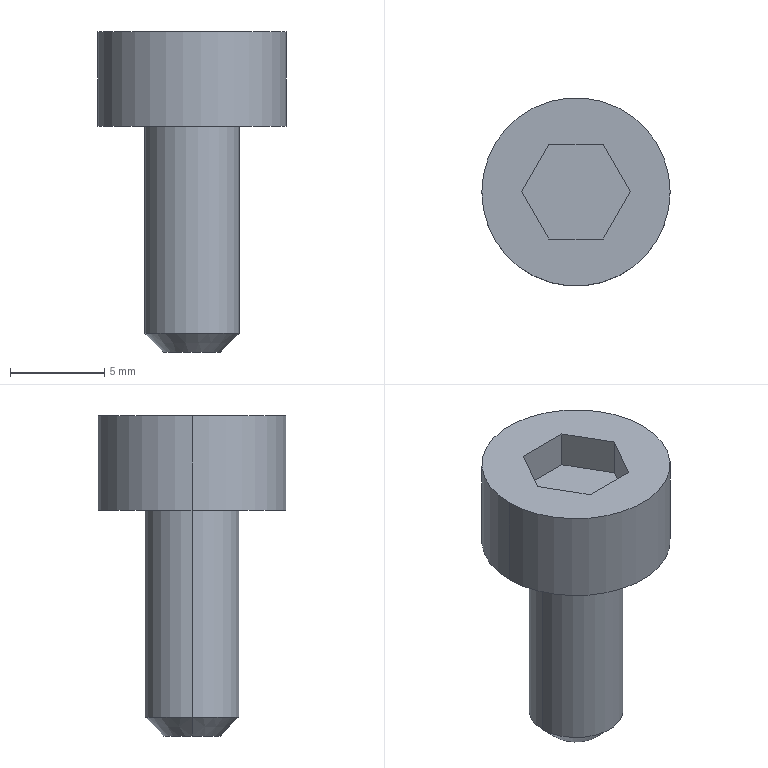Part | SolidWorks | features ICE 2, Chamfer 1, Extrusion 1 | 1 solid | 16 faces | box 10 x 10 x 17 mm | volume 578.21 mm3 | plane 10 | cylinder 4 | cone 2 | commonest cylinder face diameters 5 x2 10 x2
STEP:
#1=CARTESIAN_POINT('',(-1.5,0.,-12.));
#2=VERTEX_POINT('',#1);
#3=CARTESIAN_POINT('',(1.5,0.,-12.));
#4=VERTEX_POINT('',#3);
#5=CARTESIAN_POINT('',(0.,0.,-12.));
#6=DIRECTION('',(0.,0.,-1.));
#7=DIRECTION('',(-1.,0.,0.));
#8=AXIS2_PLACEMENT_3D('',#5,#6,#7);
#9=CIRCLE('',#8,1.5);
#10=EDGE_CURVE('',#2,#4,#9,.T.);
#11=ORIENTED_EDGE('',*,*,#10,.F.);
#12=CARTESIAN_POINT('',(-2.5,0.,-11.));
#13=VERTEX_POINT('',#12);
#14=CARTESIAN_POINT('',(-1.5,0.,-12.));
#15=DIRECTION('',(-0.7071,0.,0.7071));
#16=VECTOR('',#15,1000.);
#17=LINE('',#14,#16);
#18=EDGE_CURVE('',#2,#13,#17,.T.);
#19=ORIENTED_EDGE('',*,*,#18,.T.);
#20=CARTESIAN_POINT('',(2.5,0.,-11.));
#21=VERTEX_POINT('',#20);
#22=CARTESIAN_POINT('',(0.,0.,-11.));
#23=DIRECTION('',(0.,0.,1.));
#24=DIRECTION('',(-1.,0.,0.));
#25=AXIS2_PLACEMENT_3D('',#22,#23,#24);
#26=CIRCLE('',#25,2.5);
#27=EDGE_CURVE('',#21,#13,#26,.T.);
#28=ORIENTED_EDGE('',*,*,#27,.F.);
#29=CARTESIAN_POINT('',(1.5,0.,-12.));
#30=DIRECTION('',(0.7071,0.,0.7071));
#31=VECTOR('',#30,1000.);
#32=LINE('',#29,#31);
#33=EDGE_CURVE('',#4,#21,#32,.T.);
#34=ORIENTED_EDGE('',*,*,#33,.F.);
#35=EDGE_LOOP('',(#11,#19,#28,#34));
#36=FACE_OUTER_BOUND('',#35,.T.);
#37=CARTESIAN_POINT('',(0.,0.,-12.));
#38=DIRECTION('',(0.,0.,1.));
#39=DIRECTION('',(1.,0.,0.));
#40=AXIS2_PLACEMENT_3D('',#37,#38,#39);
#41=CONICAL_SURFACE('',#40,1.5,0.7854);
#42=ADVANCED_FACE('',(#36),#41,.T.);
#43=ORIENTED_EDGE('',*,*,#27,.T.);
#44=CARTESIAN_POINT('',(-2.5,0.,0.));
#45=VERTEX_POINT('',#44);
#46=CARTESIAN_POINT('',(-2.5,0.,-12.));
#47=DIRECTION('',(0.,0.,1.));
#48=VECTOR('',#47,1000.);
#49=LINE('',#46,#48);
#50=EDGE_CURVE('',#13,#45,#49,.T.);
#51=ORIENTED_EDGE('',*,*,#50,.T.);
#52=CARTESIAN_POINT('',(2.5,0.,0.));
#53=VERTEX_POINT('',#52);
#54=CARTESIAN_POINT('',(0.,0.,0.));
#55=DIRECTION('',(0.,0.,-1.));
#56=DIRECTION('',(-1.,0.,0.));
#57=AXIS2_PLACEMENT_3D('',#54,#55,#56);
#58=CIRCLE('',#57,2.5);
#59=EDGE_CURVE('',#45,#53,#58,.T.);
#60=ORIENTED_EDGE('',*,*,#59,.T.);
#61=CARTESIAN_POINT('',(2.5,0.,-12.));
#62=DIRECTION('',(0.,0.,1.));
#63=VECTOR('',#62,1000.);
#64=LINE('',#61,#63);
#65=EDGE_CURVE('',#21,#53,#64,.T.);
#66=ORIENTED_EDGE('',*,*,#65,.F.);
#67=EDGE_LOOP('',(#43,#51,#60,#66));
#68=FACE_OUTER_BOUND('',#67,.T.);
#69=CARTESIAN_POINT('',(0.,0.,-12.));
#70=DIRECTION('',(0.,0.,1.));
#71=DIRECTION('',(1.,0.,0.));
#72=AXIS2_PLACEMENT_3D('',#69,#70,#71);
#73=CYLINDRICAL_SURFACE('',#72,2.5);
#74=ADVANCED_FACE('',(#68),#73,.T.);
#75=CARTESIAN_POINT('',(5.,0.,5.));
#76=VERTEX_POINT('',#75);
#77=CARTESIAN_POINT('',(-5.,0.,5.));
#78=VERTEX_POINT('',#77);
#79=CARTESIAN_POINT('',(0.,0.,5.));
#80=DIRECTION('',(0.,0.,1.));
#81=DIRECTION('',(1.,0.,0.));
#82=AXIS2_PLACEMENT_3D('',#79,#80,#81);
#83=CIRCLE('',#82,5.);
#84=EDGE_CURVE('',#76,#78,#83,.T.);
#85=ORIENTED_EDGE('',*,*,#84,.F.);
#86=CARTESIAN_POINT('',(5.,0.,0.));
#87=VERTEX_POINT('',#86);
#88=CARTESIAN_POINT('',(5.,0.,5.));
#89=DIRECTION('',(0.,0.,-1.));
#90=VECTOR('',#89,1000.);
#91=LINE('',#88,#90);
#92=EDGE_CURVE('',#76,#87,#91,.T.);
#93=ORIENTED_EDGE('',*,*,#92,.T.);
#94=CARTESIAN_POINT('',(-5.,0.,0.));
#95=VERTEX_POINT('',#94);
#96=CARTESIAN_POINT('',(0.,0.,0.));
#97=DIRECTION('',(0.,0.,1.));
#98=DIRECTION('',(1.,0.,0.));
#99=AXIS2_PLACEMENT_3D('',#96,#97,#98);
#100=CIRCLE('',#99,5.);
#101=EDGE_CURVE('',#87,#95,#100,.T.);
#102=ORIENTED_EDGE('',*,*,#101,.T.);
#103=CARTESIAN_POINT('',(-5.,0.,5.));
#104=DIRECTION('',(0.,0.,-1.));
#105=VECTOR('',#104,1000.);
#106=LINE('',#103,#105);
#107=EDGE_CURVE('',#78,#95,#106,.T.);
#108=ORIENTED_EDGE('',*,*,#107,.F.);
#109=EDGE_LOOP('',(#85,#93,#102,#108));
#110=FACE_OUTER_BOUND('',#109,.T.);
#111=CARTESIAN_POINT('',(0.,0.,5.));
#112=DIRECTION('',(0.,0.,-1.));
#113=DIRECTION('',(-1.,0.,0.));
#114=AXIS2_PLACEMENT_3D('',#111,#112,#113);
#115=CYLINDRICAL_SURFACE('',#114,5.);
#116=ADVANCED_FACE('',(#110),#115,.T.);
#117=ORIENTED_EDGE('',*,*,#92,.F.);
#118=CARTESIAN_POINT('',(0.,0.,5.));
#119=DIRECTION('',(0.,0.,1.));
#120=DIRECTION('',(1.,0.,0.));
#121=AXIS2_PLACEMENT_3D('',#118,#119,#120);
#122=CIRCLE('',#121,5.);
#123=EDGE_CURVE('',#78,#76,#122,.T.);
#124=ORIENTED_EDGE('',*,*,#123,.F.);
#125=ORIENTED_EDGE('',*,*,#107,.T.);
#126=CARTESIAN_POINT('',(0.,0.,0.));
#127=DIRECTION('',(0.,0.,1.));
#128=DIRECTION('',(1.,0.,0.));
#129=AXIS2_PLACEMENT_3D('',#126,#127,#128);
#130=CIRCLE('',#129,5.);
#131=EDGE_CURVE('',#95,#87,#130,.T.);
#132=ORIENTED_EDGE('',*,*,#131,.T.);
#133=EDGE_LOOP('',(#117,#124,#125,#132));
#134=FACE_OUTER_BOUND('',#133,.T.);
#135=CARTESIAN_POINT('',(0.,0.,5.));
#136=DIRECTION('',(0.,0.,-1.));
#137=DIRECTION('',(-1.,0.,0.));
#138=AXIS2_PLACEMENT_3D('',#135,#136,#137);
#139=CYLINDRICAL_SURFACE('',#138,5.);
#140=ADVANCED_FACE('',(#134),#139,.T.);
#141=CARTESIAN_POINT('',(1.443,-2.5,5.));
#142=VERTEX_POINT('',#141);
#143=CARTESIAN_POINT('',(2.887,0.,5.));
#144=VERTEX_POINT('',#143);
#145=CARTESIAN_POINT('',(1.443,-2.5,5.));
#146=DIRECTION('',(0.5,0.866,0.));
#147=VECTOR('',#146,1000.);
#148=LINE('',#145,#147);
#149=EDGE_CURVE('',#142,#144,#148,.T.);
#150=ORIENTED_EDGE('',*,*,#149,.F.);
#151=CARTESIAN_POINT('',(-1.443,-2.5,5.));
#152=VERTEX_POINT('',#151);
#153=CARTESIAN_POINT('',(-1.443,-2.5,5.));
#154=DIRECTION('',(1.,0.,0.));
#155=VECTOR('',#154,1000.);
#156=LINE('',#153,#155);
#157=EDGE_CURVE('',#152,#142,#156,.T.);
#158=ORIENTED_EDGE('',*,*,#157,.F.);
#159=CARTESIAN_POINT('',(-2.887,0.,5.));
#160=VERTEX_POINT('',#159);
#161=CARTESIAN_POINT('',(-2.887,0.,5.));
#162=DIRECTION('',(0.5,-0.866,0.));
#163=VECTOR('',#162,1000.);
#164=LINE('',#161,#163);
#165=EDGE_CURVE('',#160,#152,#164,.T.);
#166=ORIENTED_EDGE('',*,*,#165,.F.);
#167=CARTESIAN_POINT('',(-1.443,2.5,5.));
#168=VERTEX_POINT('',#167);
#169=CARTESIAN_POINT('',(-1.443,2.5,5.));
#170=DIRECTION('',(-0.5,-0.866,0.));
#171=VECTOR('',#170,1000.);
#172=LINE('',#169,#171);
#173=EDGE_CURVE('',#168,#160,#172,.T.);
#174=ORIENTED_EDGE('',*,*,#173,.F.);
#175=CARTESIAN_POINT('',(1.443,2.5,5.));
#176=VERTEX_POINT('',#175);
#177=CARTESIAN_POINT('',(1.443,2.5,5.));
#178=DIRECTION('',(-1.,0.,0.));
#179=VECTOR('',#178,1000.);
#180=LINE('',#177,#179);
#181=EDGE_CURVE('',#176,#168,#180,.T.);
#182=ORIENTED_EDGE('',*,*,#181,.F.);
#183=CARTESIAN_POINT('',(2.887,0.,5.));
#184=DIRECTION('',(-0.5,0.866,0.));
#185=VECTOR('',#184,1000.);
#186=LINE('',#183,#185);
#187=EDGE_CURVE('',#144,#176,#186,.T.);
#188=ORIENTED_EDGE('',*,*,#187,.F.);
#189=EDGE_LOOP('',(#150,#158,#166,#174,#182,#188));
#190=FACE_BOUND('',#189,.T.);
#191=ORIENTED_EDGE('',*,*,#123,.T.);
#192=ORIENTED_EDGE('',*,*,#84,.T.);
#193=EDGE_LOOP('',(#191,#192));
#194=FACE_OUTER_BOUND('',#193,.T.);
#195=CARTESIAN_POINT('',(0.,0.,5.));
#196=DIRECTION('',(0.,0.,1.));
#197=DIRECTION('',(1.,0.,0.));
#198=AXIS2_PLACEMENT_3D('',#195,#196,#197);
#199=PLANE('',#198);
#200=ADVANCED_FACE('',(#190,#194),#199,.T.);
#201=CARTESIAN_POINT('',(0.,0.,0.));
#202=DIRECTION('',(0.,0.,-1.));
#203=DIRECTION('',(-1.,0.,0.));
#204=AXIS2_PLACEMENT_3D('',#201,#202,#203);
#205=CIRCLE('',#204,2.5);
#206=EDGE_CURVE('',#53,#45,#205,.T.);
#207=ORIENTED_EDGE('',*,*,#206,.F.);
#208=ORIENTED_EDGE('',*,*,#59,.F.);
#209=EDGE_LOOP('',(#207,#208));
#210=FACE_BOUND('',#209,.T.);
#211=ORIENTED_EDGE('',*,*,#131,.F.);
#212=ORIENTED_EDGE('',*,*,#101,.F.);
#213=EDGE_LOOP('',(#211,#212));
#214=FACE_OUTER_BOUND('',#213,.T.);
#215=CARTESIAN_POINT('',(0.,0.,0.));
#216=DIRECTION('',(0.,0.,1.));
#217=DIRECTION('',(1.,0.,0.));
#218=AXIS2_PLACEMENT_3D('',#215,#216,#217);
#219=PLANE('',#218);
#220=ADVANCED_FACE('',(#210,#214),#219,.F.);
#221=ORIENTED_EDGE('',*,*,#149,.T.);
#222=CARTESIAN_POINT('',(2.887,0.,3.));
#223=VERTEX_POINT('',#222);
#224=CARTESIAN_POINT('',(2.887,0.,3.));
#225=DIRECTION('',(0.,0.,1.));
#226=VECTOR('',#225,1000.);
#227=LINE('',#224,#226);
#228=EDGE_CURVE('',#223,#144,#227,.T.);
#229=ORIENTED_EDGE('',*,*,#228,.F.);
#230=CARTESIAN_POINT('',(1.443,-2.5,3.));
#231=VERTEX_POINT('',#230);
#232=CARTESIAN_POINT('',(1.443,-2.5,3.));
#233=DIRECTION('',(0.5,0.866,0.));
#234=VECTOR('',#233,1000.);
#235=LINE('',#232,#234);
#236=EDGE_CURVE('',#231,#223,#235,.T.);
#237=ORIENTED_EDGE('',*,*,#236,.F.);
#238=CARTESIAN_POINT('',(1.443,-2.5,3.));
#239=DIRECTION('',(0.,0.,1.));
#240=VECTOR('',#239,1000.);
#241=LINE('',#238,#240);
#242=EDGE_CURVE('',#231,#142,#241,.T.);
#243=ORIENTED_EDGE('',*,*,#242,.T.);
#244=EDGE_LOOP('',(#221,#229,#237,#243));
#245=FACE_OUTER_BOUND('',#244,.T.);
#246=CARTESIAN_POINT('',(1.443,-2.5,3.));
#247=DIRECTION('',(0.866,-0.5,0.));
#248=DIRECTION('',(0.5,0.866,0.));
#249=AXIS2_PLACEMENT_3D('',#246,#247,#248);
#250=PLANE('',#249);
#251=ADVANCED_FACE('',(#245),#250,.F.);
#252=ORIENTED_EDGE('',*,*,#157,.T.);
#253=ORIENTED_EDGE('',*,*,#242,.F.);
#254=CARTESIAN_POINT('',(-1.443,-2.5,3.));
#255=VERTEX_POINT('',#254);
#256=CARTESIAN_POINT('',(-1.443,-2.5,3.));
#257=DIRECTION('',(1.,0.,0.));
#258=VECTOR('',#257,1000.);
#259=LINE('',#256,#258);
#260=EDGE_CURVE('',#255,#231,#259,.T.);
#261=ORIENTED_EDGE('',*,*,#260,.F.);
#262=CARTESIAN_POINT('',(-1.443,-2.5,3.));
#263=DIRECTION('',(0.,0.,1.));
#264=VECTOR('',#263,1000.);
#265=LINE('',#262,#264);
#266=EDGE_CURVE('',#255,#152,#265,.T.);
#267=ORIENTED_EDGE('',*,*,#266,.T.);
#268=EDGE_LOOP('',(#252,#253,#261,#267));
#269=FACE_OUTER_BOUND('',#268,.T.);
#270=CARTESIAN_POINT('',(-1.443,-2.5,3.));
#271=DIRECTION('',(0.,-1.,0.));
#272=DIRECTION('',(1.,0.,0.));
#273=AXIS2_PLACEMENT_3D('',#270,#271,#272);
#274=PLANE('',#273);
#275=ADVANCED_FACE('',(#269),#274,.F.);
#276=ORIENTED_EDGE('',*,*,#165,.T.);
#277=ORIENTED_EDGE('',*,*,#266,.F.);
#278=CARTESIAN_POINT('',(-2.887,0.,3.));
#279=VERTEX_POINT('',#278);
#280=CARTESIAN_POINT('',(-2.887,0.,3.));
#281=DIRECTION('',(0.5,-0.866,0.));
#282=VECTOR('',#281,1000.);
#283=LINE('',#280,#282);
#284=EDGE_CURVE('',#279,#255,#283,.T.);
#285=ORIENTED_EDGE('',*,*,#284,.F.);
#286=CARTESIAN_POINT('',(-2.887,0.,3.));
#287=DIRECTION('',(0.,0.,1.));
#288=VECTOR('',#287,1000.);
#289=LINE('',#286,#288);
#290=EDGE_CURVE('',#279,#160,#289,.T.);
#291=ORIENTED_EDGE('',*,*,#290,.T.);
#292=EDGE_LOOP('',(#276,#277,#285,#291));
#293=FACE_OUTER_BOUND('',#292,.T.);
#294=CARTESIAN_POINT('',(-2.887,0.,3.));
#295=DIRECTION('',(-0.866,-0.5,0.));
#296=DIRECTION('',(0.5,-0.866,0.));
#297=AXIS2_PLACEMENT_3D('',#294,#295,#296);
#298=PLANE('',#297);
#299=ADVANCED_FACE('',(#293),#298,.F.);
#300=ORIENTED_EDGE('',*,*,#173,.T.);
#301=ORIENTED_EDGE('',*,*,#290,.F.);
#302=CARTESIAN_POINT('',(-1.443,2.5,3.));
#303=VERTEX_POINT('',#302);
#304=CARTESIAN_POINT('',(-1.443,2.5,3.));
#305=DIRECTION('',(-0.5,-0.866,0.));
#306=VECTOR('',#305,1000.);
#307=LINE('',#304,#306);
#308=EDGE_CURVE('',#303,#279,#307,.T.);
#309=ORIENTED_EDGE('',*,*,#308,.F.);
#310=CARTESIAN_POINT('',(-1.443,2.5,3.));
#311=DIRECTION('',(0.,0.,1.));
#312=VECTOR('',#311,1000.);
#313=LINE('',#310,#312);
#314=EDGE_CURVE('',#303,#168,#313,.T.);
#315=ORIENTED_EDGE('',*,*,#314,.T.);
#316=EDGE_LOOP('',(#300,#301,#309,#315));
#317=FACE_OUTER_BOUND('',#316,.T.);
#318=CARTESIAN_POINT('',(-1.443,2.5,3.));
#319=DIRECTION('',(-0.866,0.5,0.));
#320=DIRECTION('',(-0.5,-0.866,0.));
#321=AXIS2_PLACEMENT_3D('',#318,#319,#320);
#322=PLANE('',#321);
#323=ADVANCED_FACE('',(#317),#322,.F.);
#324=ORIENTED_EDGE('',*,*,#181,.T.);
#325=ORIENTED_EDGE('',*,*,#314,.F.);
#326=CARTESIAN_POINT('',(1.443,2.5,3.));
#327=VERTEX_POINT('',#326);
#328=CARTESIAN_POINT('',(1.443,2.5,3.));
#329=DIRECTION('',(-1.,0.,0.));
#330=VECTOR('',#329,1000.);
#331=LINE('',#328,#330);
#332=EDGE_CURVE('',#327,#303,#331,.T.);
#333=ORIENTED_EDGE('',*,*,#332,.F.);
#334=CARTESIAN_POINT('',(1.443,2.5,3.));
#335=DIRECTION('',(0.,0.,1.));
#336=VECTOR('',#335,1000.);
#337=LINE('',#334,#336);
#338=EDGE_CURVE('',#327,#176,#337,.T.);
#339=ORIENTED_EDGE('',*,*,#338,.T.);
#340=EDGE_LOOP('',(#324,#325,#333,#339));
#341=FACE_OUTER_BOUND('',#340,.T.);
#342=CARTESIAN_POINT('',(1.443,2.5,3.));
#343=DIRECTION('',(0.,1.,0.));
#344=DIRECTION('',(0.,0.,1.));
#345=AXIS2_PLACEMENT_3D('',#342,#343,#344);
#346=PLANE('',#345);
#347=ADVANCED_FACE('',(#341),#346,.F.);
#348=ORIENTED_EDGE('',*,*,#187,.T.);
#349=ORIENTED_EDGE('',*,*,#338,.F.);
#350=CARTESIAN_POINT('',(2.887,0.,3.));
#351=DIRECTION('',(-0.5,0.866,0.));
#352=VECTOR('',#351,1000.);
#353=LINE('',#350,#352);
#354=EDGE_CURVE('',#223,#327,#353,.T.);
#355=ORIENTED_EDGE('',*,*,#354,.F.);
#356=ORIENTED_EDGE('',*,*,#228,.T.);
#357=EDGE_LOOP('',(#348,#349,#355,#356));
#358=FACE_OUTER_BOUND('',#357,.T.);
#359=CARTESIAN_POINT('',(2.887,0.,3.));
#360=DIRECTION('',(0.866,0.5,0.));
#361=DIRECTION('',(-0.5,0.866,0.));
#362=AXIS2_PLACEMENT_3D('',#359,#360,#361);
#363=PLANE('',#362);
#364=ADVANCED_FACE('',(#358),#363,.F.);
#365=ORIENTED_EDGE('',*,*,#236,.T.);
#366=ORIENTED_EDGE('',*,*,#354,.T.);
#367=ORIENTED_EDGE('',*,*,#332,.T.);
#368=ORIENTED_EDGE('',*,*,#308,.T.);
#369=ORIENTED_EDGE('',*,*,#284,.T.);
#370=ORIENTED_EDGE('',*,*,#260,.T.);
#371=EDGE_LOOP('',(#365,#366,#367,#368,#369,#370));
#372=FACE_OUTER_BOUND('',#371,.T.);
#373=CARTESIAN_POINT('',(0.,0.,3.));
#374=DIRECTION('',(0.,0.,1.));
#375=DIRECTION('',(1.,0.,0.));
#376=AXIS2_PLACEMENT_3D('',#373,#374,#375);
#377=PLANE('',#376);
#378=ADVANCED_FACE('',(#372),#377,.T.);
#379=ORIENTED_EDGE('',*,*,#50,.F.);
#380=CARTESIAN_POINT('',(0.,0.,-11.));
#381=DIRECTION('',(0.,0.,1.));
#382=DIRECTION('',(-1.,0.,0.));
#383=AXIS2_PLACEMENT_3D('',#380,#381,#382);
#384=CIRCLE('',#383,2.5);
#385=EDGE_CURVE('',#13,#21,#384,.T.);
#386=ORIENTED_EDGE('',*,*,#385,.T.);
#387=ORIENTED_EDGE('',*,*,#65,.T.);
#388=ORIENTED_EDGE('',*,*,#206,.T.);
#389=EDGE_LOOP('',(#379,#386,#387,#388));
#390=FACE_OUTER_BOUND('',#389,.T.);
#391=CARTESIAN_POINT('',(0.,0.,-12.));
#392=DIRECTION('',(0.,0.,1.));
#393=DIRECTION('',(1.,0.,0.));
#394=AXIS2_PLACEMENT_3D('',#391,#392,#393);
#395=CYLINDRICAL_SURFACE('',#394,2.5);
#396=ADVANCED_FACE('',(#390),#395,.T.);
#397=CARTESIAN_POINT('',(0.,0.,-12.));
#398=DIRECTION('',(0.,0.,-1.));
#399=DIRECTION('',(-1.,0.,0.));
#400=AXIS2_PLACEMENT_3D('',#397,#398,#399);
#401=CIRCLE('',#400,1.5);
#402=EDGE_CURVE('',#4,#2,#401,.T.);
#403=ORIENTED_EDGE('',*,*,#402,.T.);
#404=ORIENTED_EDGE('',*,*,#10,.T.);
#405=EDGE_LOOP('',(#403,#404));
#406=FACE_OUTER_BOUND('',#405,.T.);
#407=CARTESIAN_POINT('',(0.,0.,-12.));
#408=DIRECTION('',(0.,0.,-1.));
#409=DIRECTION('',(-1.,0.,0.));
#410=AXIS2_PLACEMENT_3D('',#407,#408,#409);
#411=PLANE('',#410);
#412=ADVANCED_FACE('',(#406),#411,.T.);
#413=ORIENTED_EDGE('',*,*,#18,.F.);
#414=ORIENTED_EDGE('',*,*,#402,.F.);
#415=ORIENTED_EDGE('',*,*,#33,.T.);
#416=ORIENTED_EDGE('',*,*,#385,.F.);
#417=EDGE_LOOP('',(#413,#414,#415,#416));
#418=FACE_OUTER_BOUND('',#417,.T.);
#419=CARTESIAN_POINT('',(0.,0.,-12.));
#420=DIRECTION('',(0.,0.,1.));
#421=DIRECTION('',(1.,0.,0.));
#422=AXIS2_PLACEMENT_3D('',#419,#420,#421);
#423=CONICAL_SURFACE('',#422,1.5,0.7854);
#424=ADVANCED_FACE('',(#418),#423,.T.);
#425=CLOSED_SHELL('',(#42,#74,#116,#140,#200,#220,#251,#275,#299,#323,#347,#364,#378,#396,#412,#424));
#426=MANIFOLD_SOLID_BREP('',#425);
#427=CARTESIAN_POINT('',(0.,0.,0.));
#428=DIRECTION('',(0.,0.,1.));
#429=DIRECTION('',(1.,0.,0.));
#430=AXIS2_PLACEMENT_3D('',#427,#428,#429);
#431=(LENGTH_UNIT()NAMED_UNIT(*)SI_UNIT(.MILLI.,.METRE.));
#432=UNCERTAINTY_MEASURE_WITH_UNIT(LENGTH_MEASURE(0.00001),#431,'','');
#433=(NAMED_UNIT(*)PLANE_ANGLE_UNIT()SI_UNIT($,.RADIAN.));
#434=(NAMED_UNIT(*)SI_UNIT($,.STERADIAN.)SOLID_ANGLE_UNIT());
#435=(GEOMETRIC_REPRESENTATION_CONTEXT(3)GLOBAL_UNCERTAINTY_ASSIGNED_CONTEXT((#432))GLOBAL_UNIT_ASSIGNED_CONTEXT((#431,#433,#434))REPRESENTATION_CONTEXT('',''));
#436=ADVANCED_BREP_SHAPE_REPRESENTATION('',(#426,#430),#435);